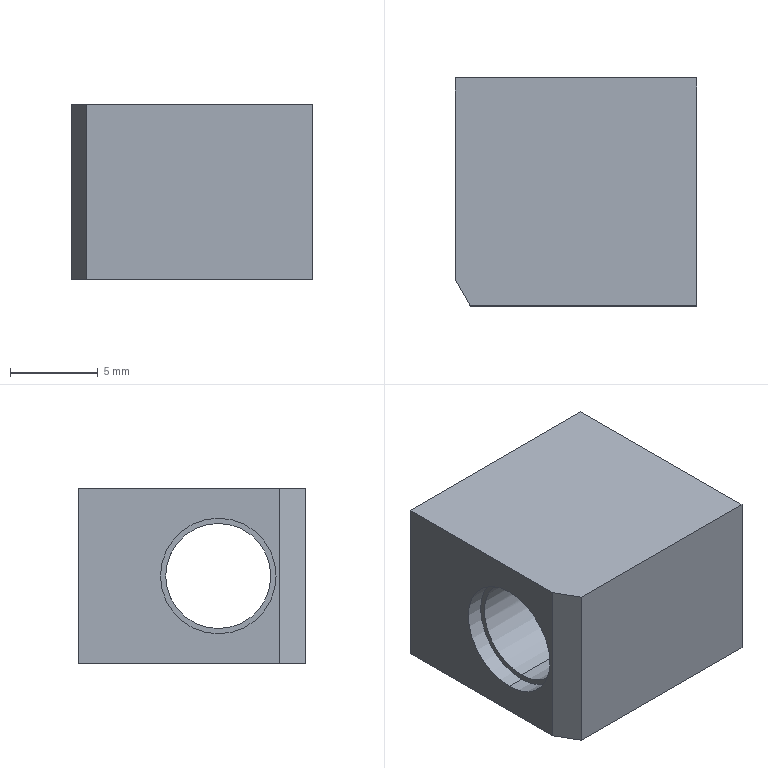Part | STEP file | 22DDSceond4trr_Default | 1 solid | 18 faces | box 13.8 x 13 x 10 mm | volume 1356 mm3 | cylinder 8 | plane 8 | cone 2 | commonest cylinder face diameters 2 x2 2.5 x2 6 x2 6.6 x2